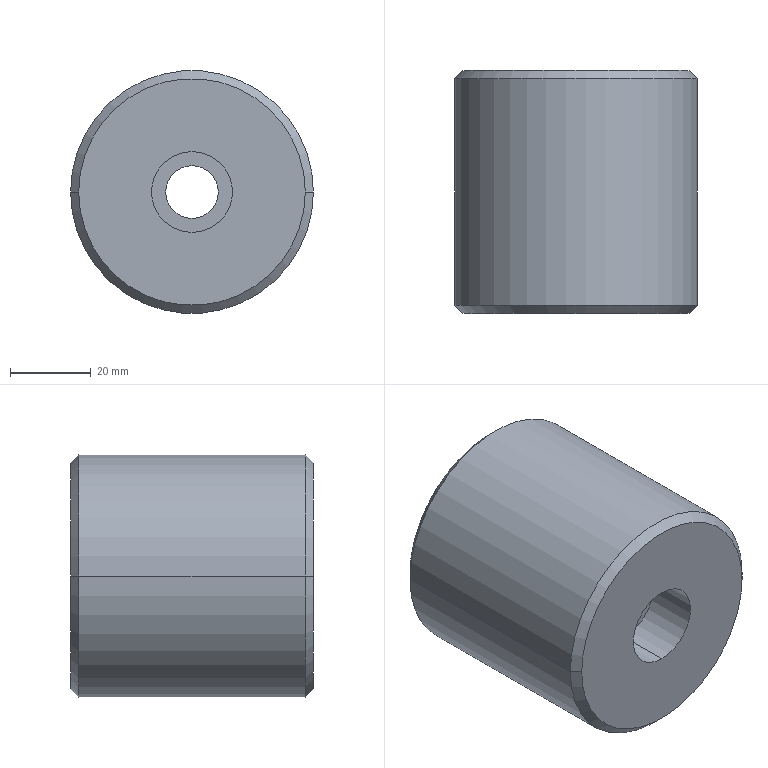Part | Creo | 1 solid | 13 faces | box 60 x 60 x 60 mm | volume 158586 mm3 | cylinder 6 | cone 4 | plane 3 | commonest cylinder face diameters 13 x2 20 x2 60 x2
STEP:
#1=CARTESIAN_POINT('',(250.,-422.005,-280.));
#2=VERTEX_POINT('',#1);
#3=CARTESIAN_POINT('',(250.,-422.005,-300.));
#4=VERTEX_POINT('',#3);
#5=CARTESIAN_POINT('',(250.,-422.005,-290.));
#6=DIRECTION('',(0.,-1.,0.));
#7=DIRECTION('',(0.,0.,1.));
#8=AXIS2_PLACEMENT_3D('',#5,#6,#7);
#9=CIRCLE('',#8,10.);
#10=EDGE_CURVE('',#2,#4,#9,.T.);
#11=ORIENTED_EDGE('',*,*,#10,.F.);
#12=CARTESIAN_POINT('',(250.,-422.005,-290.));
#13=DIRECTION('',(0.,-1.,0.));
#14=DIRECTION('',(0.,0.,-1.));
#15=AXIS2_PLACEMENT_3D('',#12,#13,#14);
#16=CIRCLE('',#15,10.);
#17=EDGE_CURVE('',#4,#2,#16,.T.);
#18=ORIENTED_EDGE('',*,*,#17,.F.);
#19=EDGE_LOOP('',(#11,#18));
#20=FACE_OUTER_BOUND('',#19,.F.);
#21=CARTESIAN_POINT('',(250.,-422.005,-283.5));
#22=VERTEX_POINT('',#21);
#23=CARTESIAN_POINT('',(256.5,-422.005,-290.));
#24=VERTEX_POINT('',#23);
#25=CARTESIAN_POINT('',(250.,-422.005,-290.));
#26=DIRECTION('',(0.,1.,0.));
#27=DIRECTION('',(0.,0.,1.));
#28=AXIS2_PLACEMENT_3D('',#25,#26,#27);
#29=CIRCLE('',#28,6.5);
#30=EDGE_CURVE('',#22,#24,#29,.T.);
#31=ORIENTED_EDGE('',*,*,#30,.F.);
#32=CARTESIAN_POINT('',(243.5,-422.005,-290.));
#33=VERTEX_POINT('',#32);
#34=CARTESIAN_POINT('',(250.,-422.005,-290.));
#35=DIRECTION('',(0.,1.,0.));
#36=DIRECTION('',(-1.,0.,0.));
#37=AXIS2_PLACEMENT_3D('',#34,#35,#36);
#38=CIRCLE('',#37,6.5);
#39=EDGE_CURVE('',#33,#22,#38,.T.);
#40=ORIENTED_EDGE('',*,*,#39,.F.);
#41=CARTESIAN_POINT('',(250.,-422.005,-290.));
#42=DIRECTION('',(0.,1.,0.));
#43=DIRECTION('',(1.,0.,0.));
#44=AXIS2_PLACEMENT_3D('',#41,#42,#43);
#45=CIRCLE('',#44,6.5);
#46=EDGE_CURVE('',#24,#33,#45,.T.);
#47=ORIENTED_EDGE('',*,*,#46,.F.);
#48=EDGE_LOOP('',(#31,#40,#47));
#49=FACE_BOUND('',#48,.F.);
#50=CARTESIAN_POINT('',(250.,-422.005,-290.));
#51=DIRECTION('',(0.,1.,0.));
#52=DIRECTION('',(0.,0.,1.));
#53=AXIS2_PLACEMENT_3D('',#50,#51,#52);
#54=PLANE('',#53);
#55=ADVANCED_FACE('',(#20,#49),#54,.F.);
#56=CARTESIAN_POINT('',(250.,-435.005,-300.));
#57=VERTEX_POINT('',#56);
#58=CARTESIAN_POINT('',(250.,-435.005,-280.));
#59=VERTEX_POINT('',#58);
#60=CARTESIAN_POINT('',(250.,-435.005,-290.));
#61=DIRECTION('',(0.,1.,0.));
#62=DIRECTION('',(0.,0.,-1.));
#63=AXIS2_PLACEMENT_3D('',#60,#61,#62);
#64=CIRCLE('',#63,10.);
#65=EDGE_CURVE('',#57,#59,#64,.T.);
#66=ORIENTED_EDGE('',*,*,#65,.T.);
#67=CARTESIAN_POINT('',(250.,-435.005,-280.));
#68=DIRECTION('',(0.,1.,0.));
#69=VECTOR('',#68,13.);
#70=LINE('',#67,#69);
#71=EDGE_CURVE('',#59,#2,#70,.T.);
#72=ORIENTED_EDGE('',*,*,#71,.T.);
#73=ORIENTED_EDGE('',*,*,#10,.T.);
#74=CARTESIAN_POINT('',(250.,-435.005,-300.));
#75=DIRECTION('',(0.,1.,0.));
#76=VECTOR('',#75,13.);
#77=LINE('',#74,#76);
#78=EDGE_CURVE('',#57,#4,#77,.T.);
#79=ORIENTED_EDGE('',*,*,#78,.F.);
#80=EDGE_LOOP('',(#66,#72,#73,#79));
#81=FACE_OUTER_BOUND('',#80,.F.);
#82=CARTESIAN_POINT('',(250.,-438.005,-290.));
#83=DIRECTION('',(0.,1.,0.));
#84=DIRECTION('',(0.,0.,1.));
#85=AXIS2_PLACEMENT_3D('',#82,#83,#84);
#86=CYLINDRICAL_SURFACE('',#85,10.);
#87=ADVANCED_FACE('',(#81),#86,.F.);
#88=CARTESIAN_POINT('',(222.,-435.005,-290.));
#89=VERTEX_POINT('',#88);
#90=CARTESIAN_POINT('',(278.,-435.005,-290.));
#91=VERTEX_POINT('',#90);
#92=CARTESIAN_POINT('',(250.,-435.005,-290.));
#93=DIRECTION('',(0.,-1.,0.));
#94=DIRECTION('',(-1.,0.,0.));
#95=AXIS2_PLACEMENT_3D('',#92,#93,#94);
#96=CIRCLE('',#95,28.);
#97=EDGE_CURVE('',#89,#91,#96,.T.);
#98=ORIENTED_EDGE('',*,*,#97,.F.);
#99=CARTESIAN_POINT('',(250.,-435.005,-290.));
#100=DIRECTION('',(0.,-1.,0.));
#101=DIRECTION('',(1.,0.,0.));
#102=AXIS2_PLACEMENT_3D('',#99,#100,#101);
#103=CIRCLE('',#102,28.);
#104=EDGE_CURVE('',#91,#89,#103,.T.);
#105=ORIENTED_EDGE('',*,*,#104,.F.);
#106=EDGE_LOOP('',(#98,#105));
#107=FACE_OUTER_BOUND('',#106,.F.);
#108=CARTESIAN_POINT('',(250.,-435.005,-290.));
#109=DIRECTION('',(0.,1.,0.));
#110=DIRECTION('',(0.,0.,1.));
#111=AXIS2_PLACEMENT_3D('',#108,#109,#110);
#112=CIRCLE('',#111,10.);
#113=EDGE_CURVE('',#59,#57,#112,.T.);
#114=ORIENTED_EDGE('',*,*,#113,.F.);
#115=ORIENTED_EDGE('',*,*,#65,.F.);
#116=EDGE_LOOP('',(#114,#115));
#117=FACE_BOUND('',#116,.F.);
#118=CARTESIAN_POINT('',(10.,-435.005,-361.));
#119=DIRECTION('',(0.,-1.,0.));
#120=DIRECTION('',(1.,0.,0.));
#121=AXIS2_PLACEMENT_3D('',#118,#119,#120);
#122=PLANE('',#121);
#123=ADVANCED_FACE('',(#107,#117),#122,.T.);
#124=ORIENTED_EDGE('',*,*,#113,.T.);
#125=ORIENTED_EDGE('',*,*,#78,.T.);
#126=ORIENTED_EDGE('',*,*,#17,.T.);
#127=ORIENTED_EDGE('',*,*,#71,.F.);
#128=EDGE_LOOP('',(#124,#125,#126,#127));
#129=FACE_OUTER_BOUND('',#128,.F.);
#130=CARTESIAN_POINT('',(250.,-438.005,-290.));
#131=DIRECTION('',(0.,1.,0.));
#132=DIRECTION('',(0.,0.,1.));
#133=AXIS2_PLACEMENT_3D('',#130,#131,#132);
#134=CYLINDRICAL_SURFACE('',#133,10.);
#135=ADVANCED_FACE('',(#129),#134,.F.);
#136=CARTESIAN_POINT('',(220.,-433.005,-290.));
#137=VERTEX_POINT('',#136);
#138=CARTESIAN_POINT('',(280.,-433.005,-290.));
#139=VERTEX_POINT('',#138);
#140=CARTESIAN_POINT('',(250.,-433.005,-290.));
#141=DIRECTION('',(0.,-1.,0.));
#142=DIRECTION('',(-1.,0.,0.));
#143=AXIS2_PLACEMENT_3D('',#140,#141,#142);
#144=CIRCLE('',#143,30.);
#145=EDGE_CURVE('',#137,#139,#144,.T.);
#146=ORIENTED_EDGE('',*,*,#145,.F.);
#147=CARTESIAN_POINT('',(222.,-435.005,-290.));
#148=DIRECTION('',(-0.7071,0.7071,0.));
#149=VECTOR('',#148,2.828);
#150=LINE('',#147,#149);
#151=EDGE_CURVE('',#89,#137,#150,.T.);
#152=ORIENTED_EDGE('',*,*,#151,.F.);
#153=ORIENTED_EDGE('',*,*,#97,.T.);
#154=CARTESIAN_POINT('',(278.,-435.005,-290.));
#155=DIRECTION('',(0.7071,0.7071,0.));
#156=VECTOR('',#155,2.828);
#157=LINE('',#154,#156);
#158=EDGE_CURVE('',#91,#139,#157,.T.);
#159=ORIENTED_EDGE('',*,*,#158,.T.);
#160=EDGE_LOOP('',(#146,#152,#153,#159));
#161=FACE_OUTER_BOUND('',#160,.F.);
#162=CARTESIAN_POINT('',(250.,-434.005,-290.));
#163=DIRECTION('',(0.,1.,0.));
#164=DIRECTION('',(-1.,0.,0.));
#165=AXIS2_PLACEMENT_3D('',#162,#163,#164);
#166=CONICAL_SURFACE('',#165,29.,45.);
#167=ADVANCED_FACE('',(#161),#166,.T.);
#168=ORIENTED_EDGE('',*,*,#145,.T.);
#169=CARTESIAN_POINT('',(280.,-377.005,-290.));
#170=VERTEX_POINT('',#169);
#171=CARTESIAN_POINT('',(280.,-377.005,-290.));
#172=DIRECTION('',(0.,-1.,0.));
#173=VECTOR('',#172,56.);
#174=LINE('',#171,#173);
#175=EDGE_CURVE('',#170,#139,#174,.T.);
#176=ORIENTED_EDGE('',*,*,#175,.F.);
#177=CARTESIAN_POINT('',(220.,-377.005,-290.));
#178=VERTEX_POINT('',#177);
#179=CARTESIAN_POINT('',(250.,-377.005,-290.));
#180=DIRECTION('',(0.,1.,0.));
#181=DIRECTION('',(1.,0.,0.));
#182=AXIS2_PLACEMENT_3D('',#179,#180,#181);
#183=CIRCLE('',#182,30.);
#184=EDGE_CURVE('',#170,#178,#183,.T.);
#185=ORIENTED_EDGE('',*,*,#184,.T.);
#186=CARTESIAN_POINT('',(220.,-377.005,-290.));
#187=DIRECTION('',(0.,-1.,0.));
#188=VECTOR('',#187,56.);
#189=LINE('',#186,#188);
#190=EDGE_CURVE('',#178,#137,#189,.T.);
#191=ORIENTED_EDGE('',*,*,#190,.T.);
#192=EDGE_LOOP('',(#168,#176,#185,#191));
#193=FACE_OUTER_BOUND('',#192,.F.);
#194=CARTESIAN_POINT('',(250.,-375.005,-290.));
#195=DIRECTION('',(0.,-1.,0.));
#196=DIRECTION('',(1.,0.,0.));
#197=AXIS2_PLACEMENT_3D('',#194,#195,#196);
#198=CYLINDRICAL_SURFACE('',#197,30.);
#199=ADVANCED_FACE('',(#193),#198,.T.);
#200=CARTESIAN_POINT('',(250.,-433.005,-290.));
#201=DIRECTION('',(0.,-1.,0.));
#202=DIRECTION('',(1.,0.,0.));
#203=AXIS2_PLACEMENT_3D('',#200,#201,#202);
#204=CIRCLE('',#203,30.);
#205=EDGE_CURVE('',#139,#137,#204,.T.);
#206=ORIENTED_EDGE('',*,*,#205,.T.);
#207=ORIENTED_EDGE('',*,*,#190,.F.);
#208=CARTESIAN_POINT('',(250.,-377.005,-290.));
#209=DIRECTION('',(0.,1.,0.));
#210=DIRECTION('',(-1.,0.,0.));
#211=AXIS2_PLACEMENT_3D('',#208,#209,#210);
#212=CIRCLE('',#211,30.);
#213=EDGE_CURVE('',#178,#170,#212,.T.);
#214=ORIENTED_EDGE('',*,*,#213,.T.);
#215=ORIENTED_EDGE('',*,*,#175,.T.);
#216=EDGE_LOOP('',(#206,#207,#214,#215));
#217=FACE_OUTER_BOUND('',#216,.F.);
#218=CARTESIAN_POINT('',(250.,-375.005,-290.));
#219=DIRECTION('',(0.,-1.,0.));
#220=DIRECTION('',(1.,0.,0.));
#221=AXIS2_PLACEMENT_3D('',#218,#219,#220);
#222=CYLINDRICAL_SURFACE('',#221,30.);
#223=ADVANCED_FACE('',(#217),#222,.T.);
#224=ORIENTED_EDGE('',*,*,#205,.F.);
#225=ORIENTED_EDGE('',*,*,#158,.F.);
#226=ORIENTED_EDGE('',*,*,#104,.T.);
#227=ORIENTED_EDGE('',*,*,#151,.T.);
#228=EDGE_LOOP('',(#224,#225,#226,#227));
#229=FACE_OUTER_BOUND('',#228,.F.);
#230=CARTESIAN_POINT('',(250.,-434.005,-290.));
#231=DIRECTION('',(0.,1.,0.));
#232=DIRECTION('',(-1.,0.,0.));
#233=AXIS2_PLACEMENT_3D('',#230,#231,#232);
#234=CONICAL_SURFACE('',#233,29.,45.);
#235=ADVANCED_FACE('',(#229),#234,.T.);
#236=ORIENTED_EDGE('',*,*,#213,.F.);
#237=CARTESIAN_POINT('',(222.,-375.005,-290.));
#238=VERTEX_POINT('',#237);
#239=CARTESIAN_POINT('',(222.,-375.005,-290.));
#240=DIRECTION('',(-0.7071,-0.7071,0.));
#241=VECTOR('',#240,2.828);
#242=LINE('',#239,#241);
#243=EDGE_CURVE('',#238,#178,#242,.T.);
#244=ORIENTED_EDGE('',*,*,#243,.F.);
#245=CARTESIAN_POINT('',(278.,-375.005,-290.));
#246=VERTEX_POINT('',#245);
#247=CARTESIAN_POINT('',(250.,-375.005,-290.));
#248=DIRECTION('',(0.,1.,0.));
#249=DIRECTION('',(-1.,0.,0.));
#250=AXIS2_PLACEMENT_3D('',#247,#248,#249);
#251=CIRCLE('',#250,28.);
#252=EDGE_CURVE('',#238,#246,#251,.T.);
#253=ORIENTED_EDGE('',*,*,#252,.T.);
#254=CARTESIAN_POINT('',(278.,-375.005,-290.));
#255=DIRECTION('',(0.7071,-0.7071,0.));
#256=VECTOR('',#255,2.828);
#257=LINE('',#254,#256);
#258=EDGE_CURVE('',#246,#170,#257,.T.);
#259=ORIENTED_EDGE('',*,*,#258,.T.);
#260=EDGE_LOOP('',(#236,#244,#253,#259));
#261=FACE_OUTER_BOUND('',#260,.F.);
#262=CARTESIAN_POINT('',(250.,-376.005,-290.));
#263=DIRECTION('',(0.,-1.,0.));
#264=DIRECTION('',(-1.,0.,0.));
#265=AXIS2_PLACEMENT_3D('',#262,#263,#264);
#266=CONICAL_SURFACE('',#265,29.,45.);
#267=ADVANCED_FACE('',(#261),#266,.T.);
#268=ORIENTED_EDGE('',*,*,#184,.F.);
#269=ORIENTED_EDGE('',*,*,#258,.F.);
#270=CARTESIAN_POINT('',(250.,-375.005,-290.));
#271=DIRECTION('',(0.,1.,0.));
#272=DIRECTION('',(1.,0.,0.));
#273=AXIS2_PLACEMENT_3D('',#270,#271,#272);
#274=CIRCLE('',#273,28.);
#275=EDGE_CURVE('',#246,#238,#274,.T.);
#276=ORIENTED_EDGE('',*,*,#275,.T.);
#277=ORIENTED_EDGE('',*,*,#243,.T.);
#278=EDGE_LOOP('',(#268,#269,#276,#277));
#279=FACE_OUTER_BOUND('',#278,.F.);
#280=CARTESIAN_POINT('',(250.,-376.005,-290.));
#281=DIRECTION('',(0.,-1.,0.));
#282=DIRECTION('',(-1.,0.,0.));
#283=AXIS2_PLACEMENT_3D('',#280,#281,#282);
#284=CONICAL_SURFACE('',#283,29.,45.);
#285=ADVANCED_FACE('',(#279),#284,.T.);
#286=ORIENTED_EDGE('',*,*,#252,.F.);
#287=ORIENTED_EDGE('',*,*,#275,.F.);
#288=EDGE_LOOP('',(#286,#287));
#289=FACE_OUTER_BOUND('',#288,.F.);
#290=CARTESIAN_POINT('',(256.5,-375.005,-290.));
#291=VERTEX_POINT('',#290);
#292=CARTESIAN_POINT('',(243.5,-375.005,-290.));
#293=VERTEX_POINT('',#292);
#294=CARTESIAN_POINT('',(250.,-375.005,-290.));
#295=DIRECTION('',(0.,-1.,0.));
#296=DIRECTION('',(1.,0.,0.));
#297=AXIS2_PLACEMENT_3D('',#294,#295,#296);
#298=CIRCLE('',#297,6.5);
#299=EDGE_CURVE('',#291,#293,#298,.T.);
#300=ORIENTED_EDGE('',*,*,#299,.F.);
#301=CARTESIAN_POINT('',(250.,-375.005,-290.));
#302=DIRECTION('',(0.,-1.,0.));
#303=DIRECTION('',(-1.,0.,0.));
#304=AXIS2_PLACEMENT_3D('',#301,#302,#303);
#305=CIRCLE('',#304,6.5);
#306=EDGE_CURVE('',#293,#291,#305,.T.);
#307=ORIENTED_EDGE('',*,*,#306,.F.);
#308=EDGE_LOOP('',(#300,#307));
#309=FACE_BOUND('',#308,.F.);
#310=CARTESIAN_POINT('',(10.,-375.005,-361.));
#311=DIRECTION('',(0.,-1.,0.));
#312=DIRECTION('',(1.,0.,0.));
#313=AXIS2_PLACEMENT_3D('',#310,#311,#312);
#314=PLANE('',#313);
#315=ADVANCED_FACE('',(#289,#309),#314,.F.);
#316=ORIENTED_EDGE('',*,*,#39,.T.);
#317=ORIENTED_EDGE('',*,*,#30,.T.);
#318=CARTESIAN_POINT('',(256.5,-422.005,-290.));
#319=DIRECTION('',(0.,1.,0.));
#320=VECTOR('',#319,47.);
#321=LINE('',#318,#320);
#322=EDGE_CURVE('',#24,#291,#321,.T.);
#323=ORIENTED_EDGE('',*,*,#322,.T.);
#324=ORIENTED_EDGE('',*,*,#299,.T.);
#325=CARTESIAN_POINT('',(243.5,-422.005,-290.));
#326=DIRECTION('',(0.,1.,0.));
#327=VECTOR('',#326,47.);
#328=LINE('',#325,#327);
#329=EDGE_CURVE('',#33,#293,#328,.T.);
#330=ORIENTED_EDGE('',*,*,#329,.F.);
#331=EDGE_LOOP('',(#316,#317,#323,#324,#330));
#332=FACE_OUTER_BOUND('',#331,.F.);
#333=CARTESIAN_POINT('',(250.,-447.005,-290.));
#334=DIRECTION('',(0.,1.,0.));
#335=DIRECTION('',(1.,0.,0.));
#336=AXIS2_PLACEMENT_3D('',#333,#334,#335);
#337=CYLINDRICAL_SURFACE('',#336,6.5);
#338=ADVANCED_FACE('',(#332),#337,.F.);
#339=ORIENTED_EDGE('',*,*,#46,.T.);
#340=ORIENTED_EDGE('',*,*,#329,.T.);
#341=ORIENTED_EDGE('',*,*,#306,.T.);
#342=ORIENTED_EDGE('',*,*,#322,.F.);
#343=EDGE_LOOP('',(#339,#340,#341,#342));
#344=FACE_OUTER_BOUND('',#343,.F.);
#345=CARTESIAN_POINT('',(250.,-447.005,-290.));
#346=DIRECTION('',(0.,1.,0.));
#347=DIRECTION('',(1.,0.,0.));
#348=AXIS2_PLACEMENT_3D('',#345,#346,#347);
#349=CYLINDRICAL_SURFACE('',#348,6.5);
#350=ADVANCED_FACE('',(#344),#349,.F.);
#351=CLOSED_SHELL('',(#55,#87,#123,#135,#167,#199,#223,#235,#267,#285,#315,#338,#350));
#352=MANIFOLD_SOLID_BREP('',#351);
#353=(LENGTH_UNIT()NAMED_UNIT(*)SI_UNIT(.MILLI.,.METRE.));
#354=UNCERTAINTY_MEASURE_WITH_UNIT(LENGTH_MEASURE(0.01039),#353,'','');
#355=(NAMED_UNIT(*)PLANE_ANGLE_UNIT()SI_UNIT($,.RADIAN.));
#356=PLANE_ANGLE_MEASURE_WITH_UNIT(PLANE_ANGLE_MEASURE(0.01745),#355);
#357=(CONVERSION_BASED_UNIT('DEGREE',#356)NAMED_UNIT(*)PLANE_ANGLE_UNIT());
#358=(NAMED_UNIT(*)SI_UNIT($,.STERADIAN.)SOLID_ANGLE_UNIT());
#359=(GEOMETRIC_REPRESENTATION_CONTEXT(3)GLOBAL_UNCERTAINTY_ASSIGNED_CONTEXT((#354))GLOBAL_UNIT_ASSIGNED_CONTEXT((#353,#357,#358))REPRESENTATION_CONTEXT('',''));
#360=ADVANCED_BREP_SHAPE_REPRESENTATION('',(#352),#359);